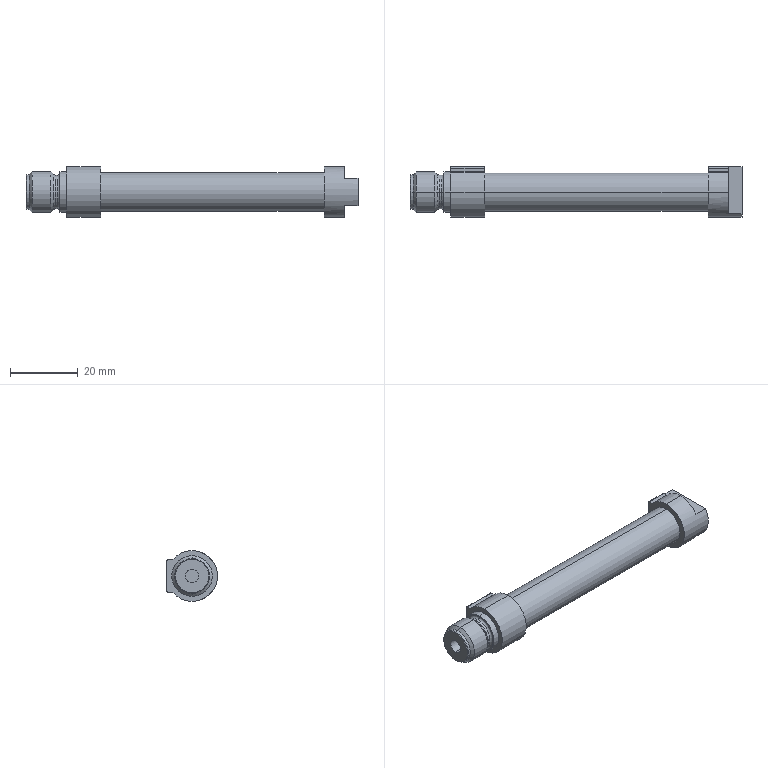Part | STEP file | PN_0051 | 1 solid | 69 faces | box 98 x 15 x 15 mm | volume 7309 mm3 | cylinder 33 | plane 20 | cone 12 | torus 4 | commonest cylinder face diameters 15 x6 0.6 x4 0.8 x4 4.134 x4 10 x4 12 x4